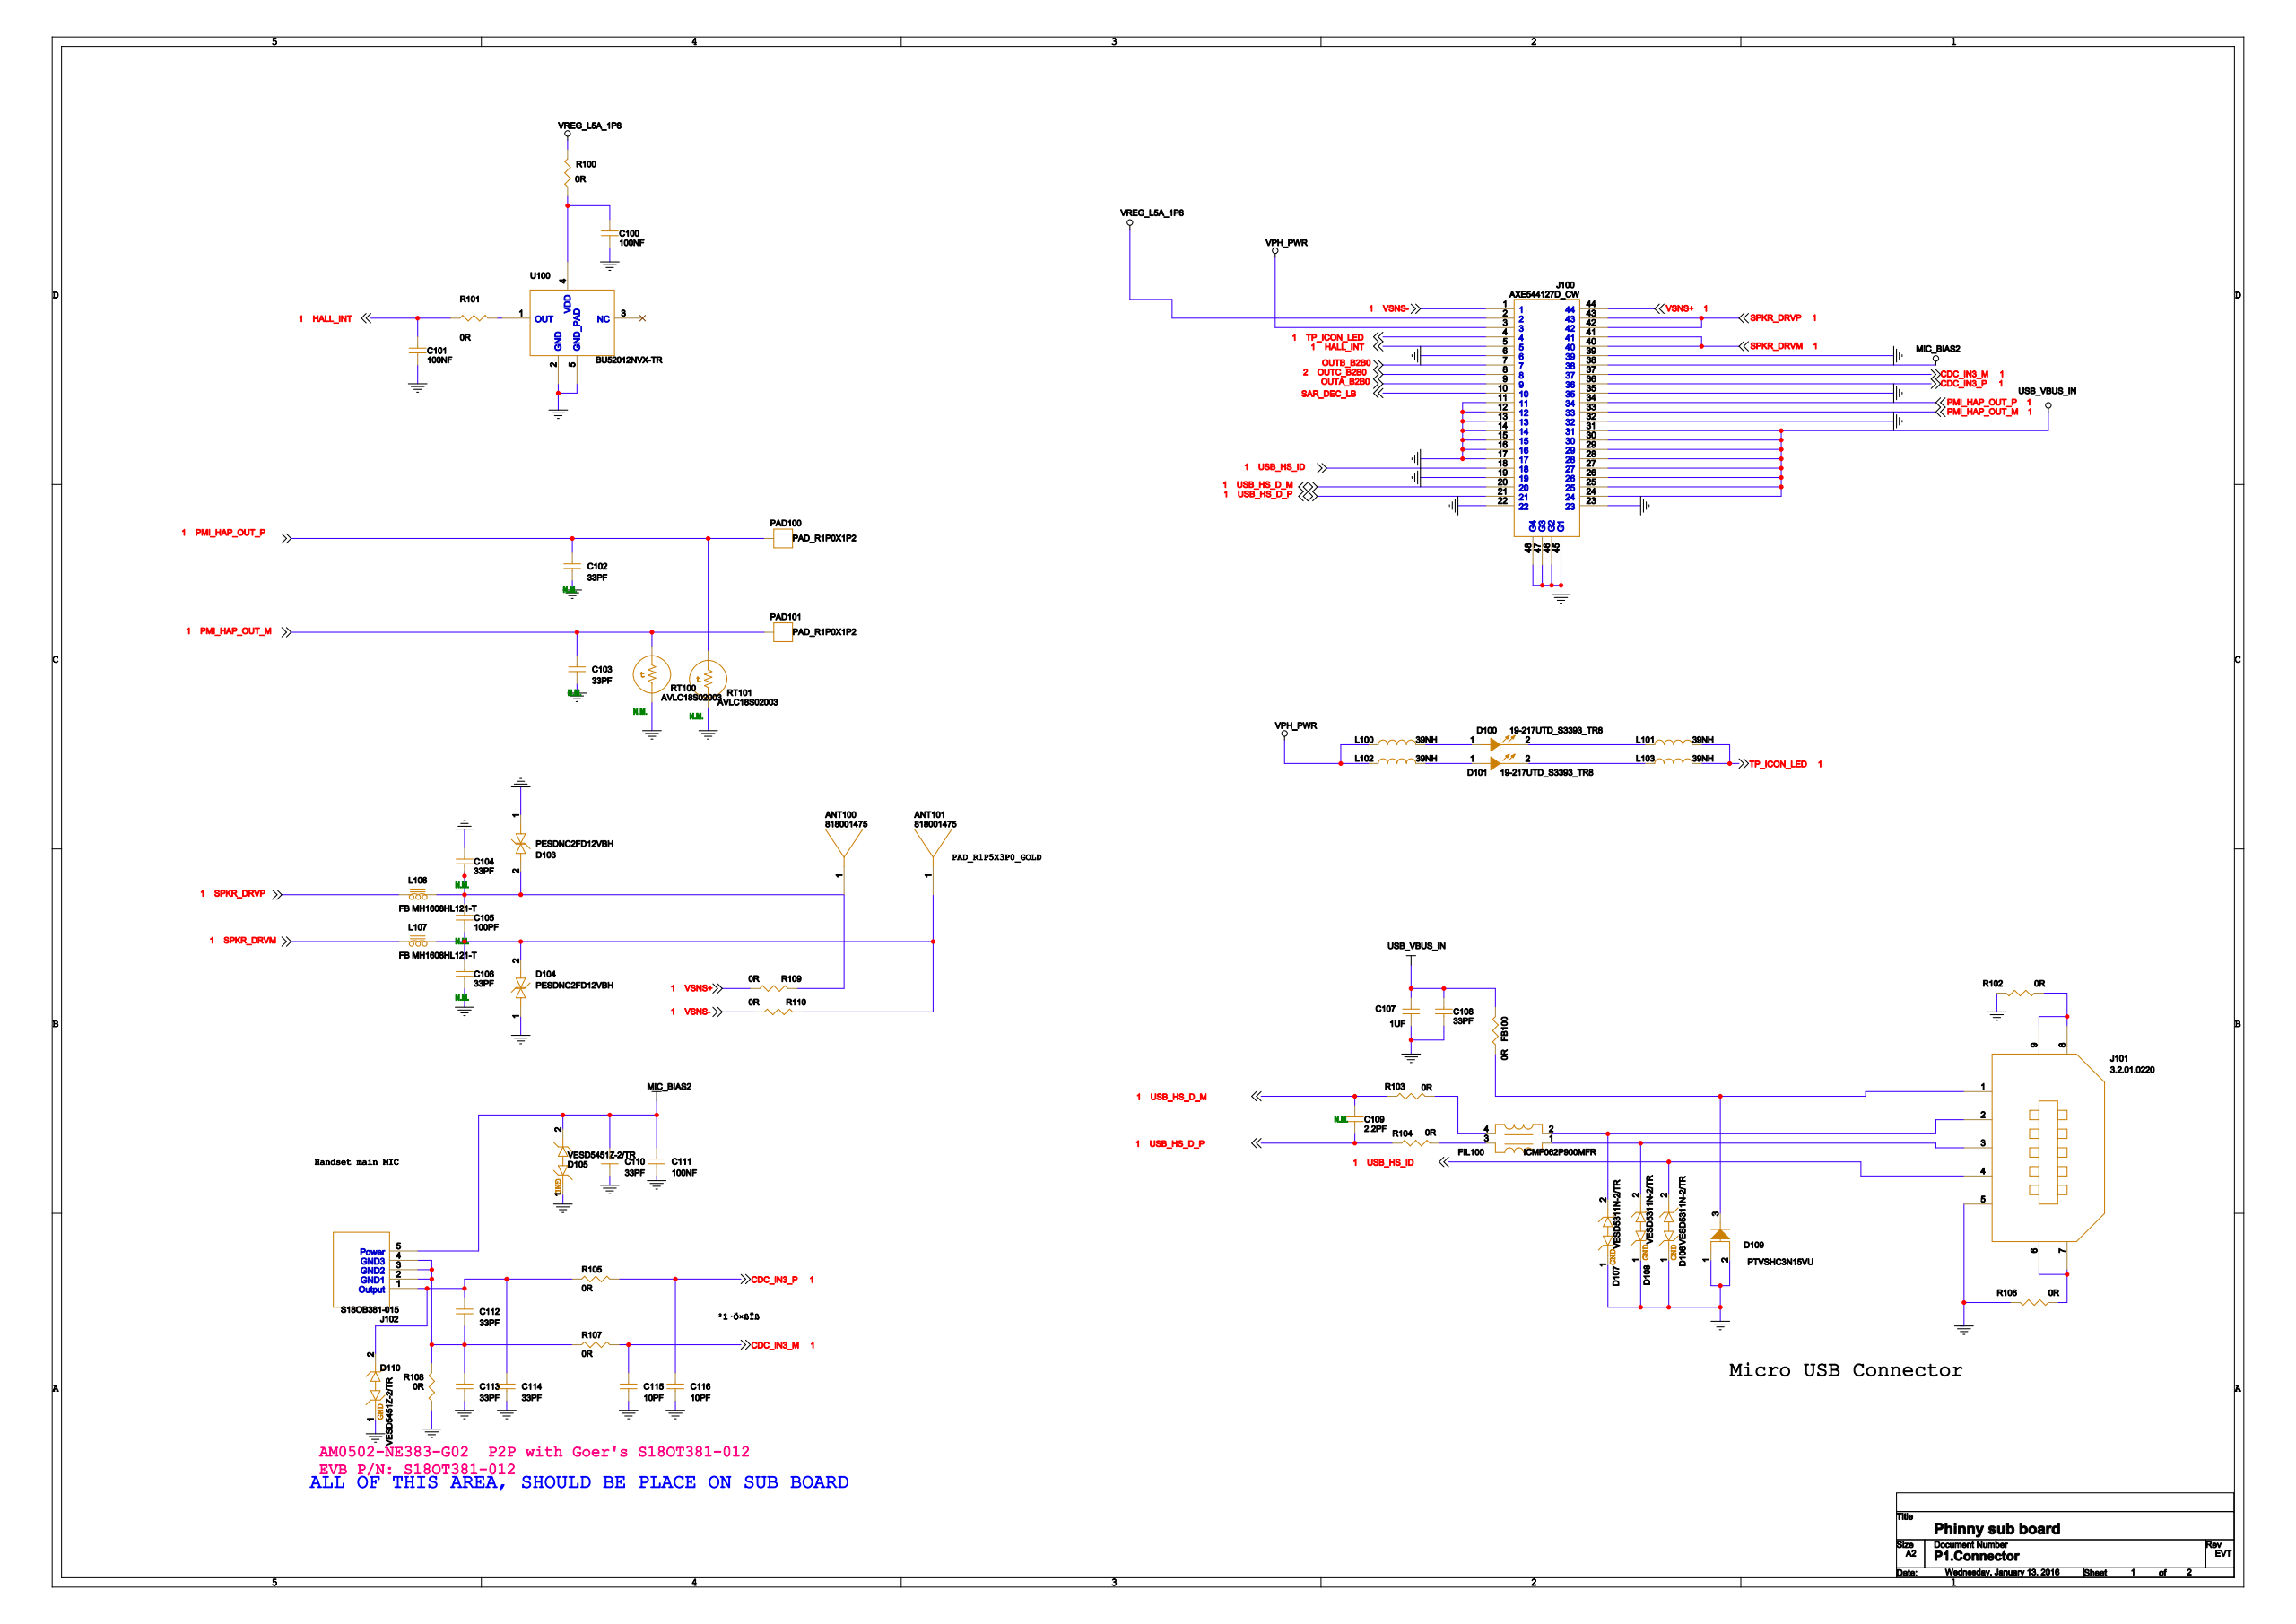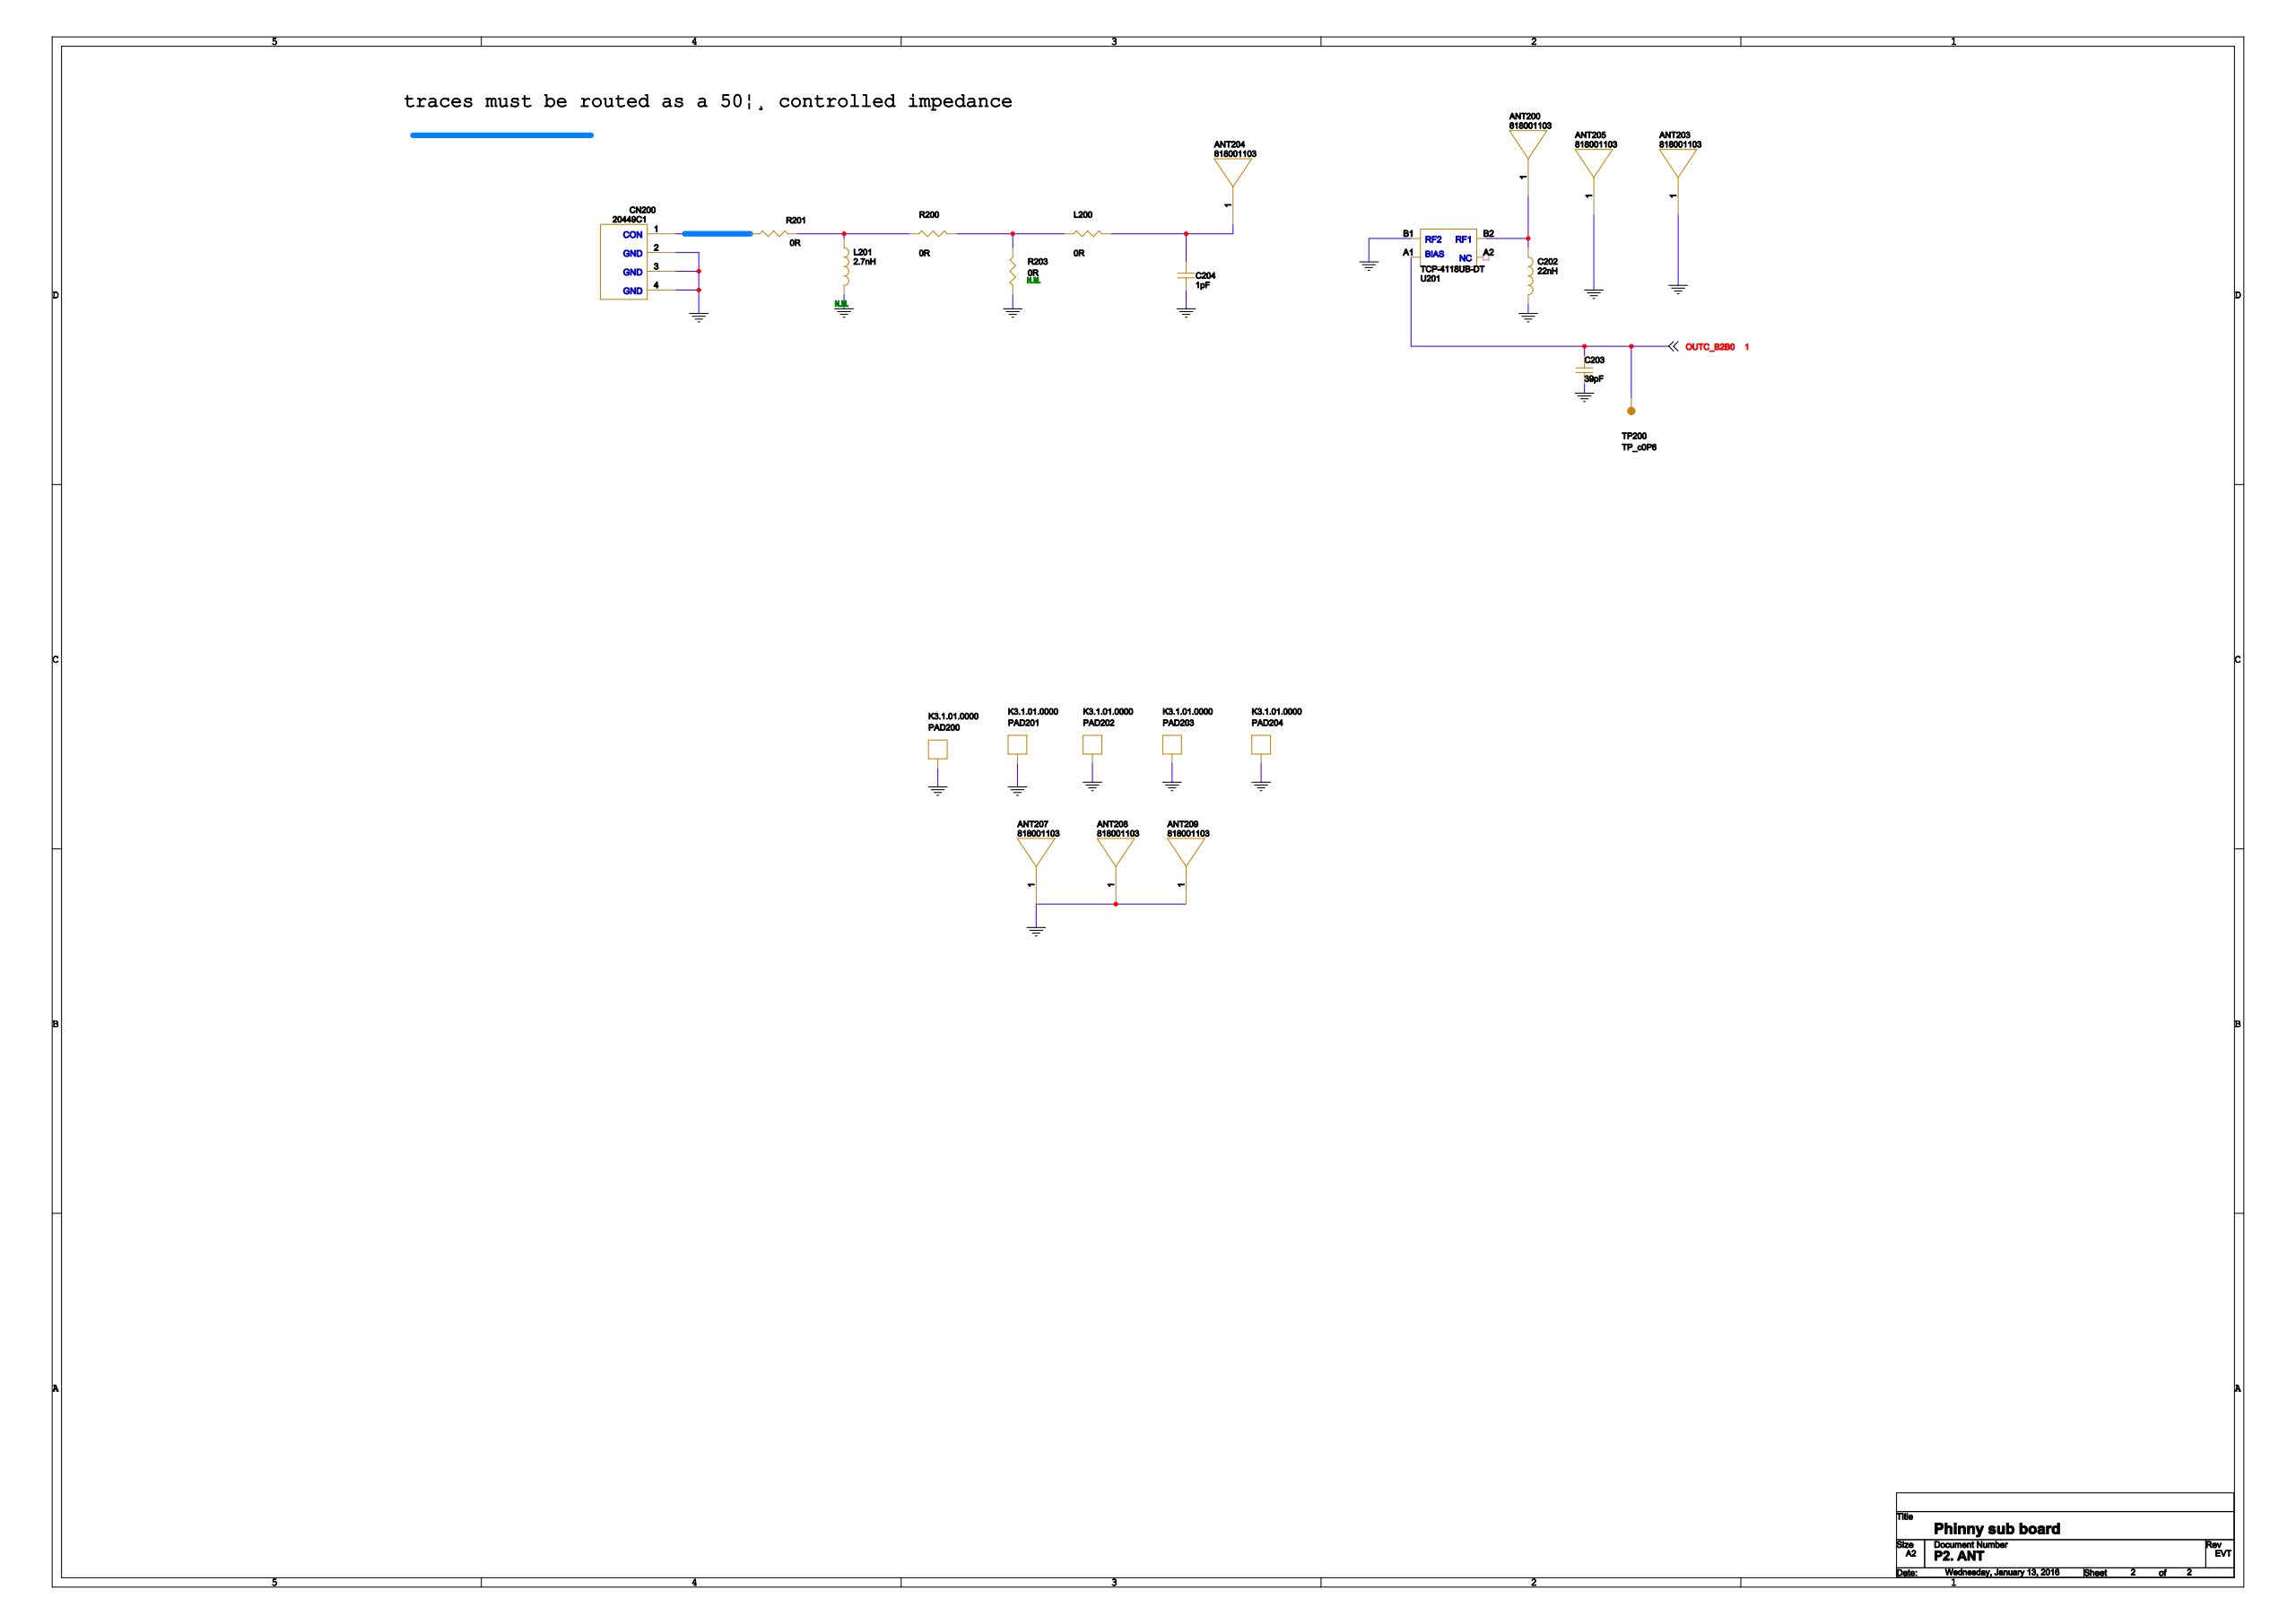Circuit board | Cadence Allegro | 79 parts | 44 nets
Bill of materials:
SYM_NAME,COMP_DEVICE_TYPE,COMP_VALUE,COMP_TOL,COMP_CLASS,REFDES
PIN_ANT_818001475,PIN_ANT_PIN_ANT_818001475_81800,818001475,,IC,ANT100
PIN_ANT_818001475,PIN_ANT_PIN_ANT_818001475_81800,818001475,,IC,ANT101
PIN_ANT_818001103,PIN_ANT_PIN_ANT_818001103_81800,818001103,,IC,ANT200
PIN_ANT_818001103,PIN_ANT_PIN_ANT_818001103_81800,818001103,,IC,ANT203
PIN_ANT_818001103,PIN_ANT_PIN_ANT_818001103_81800,818001103,,IC,ANT204
PIN_ANT_818001103,PIN_ANT_PIN_ANT_818001103_81800,818001103,,IC,ANT205
PIN_ANT_818001103,PIN_ANT_PIN_ANT_818001103_81800,818001103,,IC,ANT207
PIN_ANT_818001103,PIN_ANT_PIN_ANT_818001103_81800,818001103,,IC,ANT208
PIN_ANT_818001103,PIN_ANT_PIN_ANT_818001103_81800,818001103,,IC,ANT209
C0201,C_C0201_100NF,100NF,,IC,C100
C0201,C_C0201_100NF,100NF,,IC,C101
C0201,C_C0201_33PF,33PF,,IC,C102
C0201,C_C0201_33PF,33PF,,IC,C103
C0201,C_C0201_33PF,33PF,,IC,C104
C0201,C_C0201_100PF,100PF,,IC,C105
C0201,C_C0201_33PF,33PF,,IC,C106
C0603,C_C0603_1UF,1UF,,IC,C107
C0201,C_C0201_33PF,33PF,,IC,C108
C0201,C_C0201_2.2PF,2.2PF,,IC,C109
C0201,C_C0201_33PF,33PF,,IC,C110
C0201,C_C0201_100NF,100NF,,IC,C111
C0201,C_C0201_33PF,33PF,,IC,C112
C0201,C_C0201_33PF,33PF,,IC,C113
C0201,C_C0201_33PF,33PF,,IC,C114
C0201,C_C0201_10PF,10PF,,IC,C115
C0201,C_C0201_10PF,10PF,,IC,C116
L0402,L_L0402_22NH,22nH,,IC,C202
C0201,C_C0201_39PF,39pF,,IC,C203
C0402,C_C0402_1PF,1pF,,IC,C204
RF_20449C1,20449C1_RF_20449C1_20449C1,20449C1,,IC,CN200
19-217UTD_S3393_TR8,LED_SINGLE_19-217UTD_S3393_TR8_,19-217UTD_S3393_TR8,,IC,D100
19-217UTD_S3393_TR8,LED_SINGLE_19-217UTD_S3393_TR8_,19-217UTD_S3393_TR8,,IC,D101
DFN1006-2L,TVS_DOUBLE_N_DFN1006-2L_PESDNC2,PESDNC2FD12VBH,,IC,D103
DFN1006-2L,TVS_DOUBLE_N_DFN1006-2L_PESDNC2,PESDNC2FD12VBH,,IC,D104
DFN0603-2L,TVS_DOUBLE_DFN0603-2L_VESD5451Z,VESD5451Z-2/TR,,IC,D105
DFN1006-2,TVS_DOUBLE_DFN1006-2_VESD5311N-,VESD5311N-2/TR,,IC,D106
DFN1006-2,TVS_DOUBLE_DFN1006-2_VESD5311N-,VESD5311N-2/TR,,IC,D107
DFN1006-2,TVS_DOUBLE_DFN1006-2_VESD5311N-,VESD5311N-2/TR,,IC,D108
DFN2X2-3L,PTVS12VU1UPA_DFN2X2-3L_PTVSHC3N,PTVSHC3N15VU,,IC,D109
DFN0603-2L,TVS_DOUBLE_DFN0603-2L_VESD5451Z,VESD5451Z-2/TR,,IC,D110
R0603,R_R0603_0R,0R,,IC,FB100
EMI4_0P87X0P67X0P62_INNOCHIPS,ICMF062P900MFR_EMI4_0P87X0P67X0,ICMF062P900MFR,,IC,FIL100
BTB_AXE544124_CW,AXE544124_CW_BTB_AXE544124_CW_A,AXE544127D_CW,,IC,J100
USB_3_2_01_0220,UB005-17323A51_USB_3_2_01_0220_,3.2.01.0220,,IC,J101
S18OB381-015,AM0502B_NE383_M02_S18OB381-015_,S18OB381-015,,IC,J102
L0201,L_L0201_39NH,39NH,,IC,L100
L0201,L_L0201_39NH,39NH,,IC,L101
L0201,L_L0201_39NH,39NH,,IC,L102
L0201,L_L0201_39NH,39NH,,IC,L103
L0603,FB_L0603_FB MH1608HL121-T,FB MH1608HL121-T,,IC,L106
L0603,FB_L0603_FB MH1608HL121-T,FB MH1608HL121-T,,IC,L107
R0402,R_R0402_0R,0R,,IC,L200
L0402,L_L0402_2.7NH,2.7nH,,IC,L201
PAD_R1P0X1P2,PAD_R_PAD_R1P0X1P2_PAD_R1P0X1P2,PAD_R1P0X1P2,,IC,PAD100
PAD_R1P0X1P2,PAD_R_PAD_R1P0X1P2_PAD_R1P0X1P2,PAD_R1P0X1P2,,IC,PAD101
PIN_GND_5M89A463VK,PAD_R_PIN_GND_5M89A463VK_K3.1.0,K3.1.01.0000,,IC,PAD200
PIN_GND_5M89A463VK,PAD_R_PIN_GND_5M89A463VK_K3.1.0,K3.1.01.0000,,IC,PAD201
PIN_GND_5M89A463VK,PAD_R_PIN_GND_5M89A463VK_K3.1.0,K3.1.01.0000,,IC,PAD202
PIN_GND_5M89A463VK,PAD_R_PIN_GND_5M89A463VK_K3.1.0,K3.1.01.0000,,IC,PAD203
PIN_GND_5M89A463VK,PAD_R_PIN_GND_5M89A463VK_K3.1.0,K3.1.01.0000,,IC,PAD204
R0201,R_R0201_0R,0R,,IC,R100
R0201,R_R0201_0R,0R,,IC,R101
R0603,R_R0603_0R,0R,,IC,R102
R0201,R_R0201_0R,0R,,IC,R103
R0201,R_R0201_0R,0R,,IC,R104
R0402,R_R0402_0R,0R,,IC,R105
R0603,R_R0603_0R,0R,,IC,R106
R0402,R_R0402_0R,0R,,IC,R107
R0201,R_R0201_0R,0R,,IC,R108
R0201,R_R0201_0R,0R,,IC,R109
R0201,R_R0201_0R,0R,,IC,R110
R0402,R_R0402_0R,0R,,IC,R200
R0402,R_R0402_0R,0R,,IC,R201
R0402,R_R0402_0R,0R,,IC,R203
R0402,RT_R0402_AVLC18S02003,AVLC18S02003,,IC,RT100
R0402,RT_R0402_AVLC18S02003,AVLC18S02003,,IC,RT101
TP_C0P6,TP_TP_C0P6_TP_C0P6,TP_c0P6,,IC,TP200
SSON004X1216,BU52012NVX-TR_SSON004X1216_BU52,BU52012NVX-TR,,IC,U100
WLCSP4_0P609X0P626X0P445,TCP-4112UB-DT_WLCSP4_0P609X0P62,TCP-4118UB-DT,,IC,U201
Netlist (net: part-pin ...):
N18809773: ANT204-1 C204-1 L200-2
GND: ANT203-1 ANT205-1 ANT207-1 ANT208-1 ANT209-1 C100-2 C101-2 C102-2 C103-2 C104-1 C106-2 C107-2 C108-2 C110-2 C111-2 C113-2 C114-2 C115-2 C116-2 C202-2 C203-1 C204-2 CN200-2 CN200-3 CN200-4 D103-1 D104-1 D105-1 D106-1 D107-1 D108-1 D109-1 D109-2 D110-1 J100-6 J100-11 J100-12 J100-13 J100-14 J100-15 J100-16 J100-17 J100-19 J100-22 J100-23 J100-32 J100-35 J100-39 J100-45 J100-46 J100-47 J100-48 J101-5 L201-2 PAD200-1 PAD201-1 PAD202-1 PAD203-1 PAD204-1 R102-2 R106-2 R108-1 R203-1 RT100-2 RT101-2 U100-2 U100-5 U201-B1
OUTC_B2B0: C203-2 J100-8 TP200-1 U201-A1
N18733889: ANT200-1 C202-1 U201-B2
N18857865: D100-1 L100-2
N18857871: D100-2 L101-1
N18857821: D101-1 L102-2
N18857789: D101-2 L103-1
USB_VBUS_IN: C107-1 C108-1 FB100-2 J100-24 J100-25 J100-26 J100-27 J100-28 J100-29 J100-30 J100-31
USB_HS_D_M: C109-1 J100-20 R103-1
USB_HS_D_P: C109-2 J100-21 R104-1
N18730979: L201-1 R200-1 R201-2
N18846591: ANT100-1 C104-2 C105-1 D103-2 L106-2 R109-1
N18846541: ANT101-1 C105-2 C106-1 D104-2 L107-2 R110-1
MIC_BIAS2: C110-1 C111-1 D105-2 J100-38 J102-5
N18845484: C112-1 C114-1 D110-2 J102-1 R105-1
USB_HS_ID: D106-2 J100-18 J101-4
N18858335: D107-2 FIL100-2 J101-2
N18858337: D108-2 FIL100-1 J101-3
N18858379: D109-3 FB100-1 J101-1
N18858430: FIL100-3 R104-2
N18858369: FIL100-4 R103-2
VSNS-: J100-1 R110-2
SAR_DEC_LB: J100-10
VREG_L5A_1P8: J100-2 R100-2
VPH_PWR: J100-3 L100-1 L102-1
PMI_HAP_OUT_M: C103-1 J100-33 PAD101-1 RT100-1
PMI_HAP_OUT_P: C102-1 J100-34 PAD100-1 RT101-1
CDC_IN3_P: C116-1 J100-36 R105-2
CDC_IN3_M: C115-1 J100-37 R107-2
TP_ICON_LED: J100-4 L101-2 L103-2
SPKR_DRVM: J100-40 J100-41 L107-1
SPKR_DRVP: J100-42 J100-43 L106-1
VSNS+: J100-44 R109-2
HALL_INT: C101-1 J100-5 R101-1
OUTB_B2B0: J100-7
OUTA_B2B0: J100-9
N18858549: J101-6 J101-7 R106-1
N18858573: J101-8 J101-9 R102-1
N18845498: C112-2 C113-1 J102-2 J102-3 J102-4 R107-1 R108-2
N18845992: C100-1 R100-1 U100-4
N18731084: CN200-1 R201-1
N18846000: R101-2 U100-1
N18870750: L200-1 R200-2 R203-2